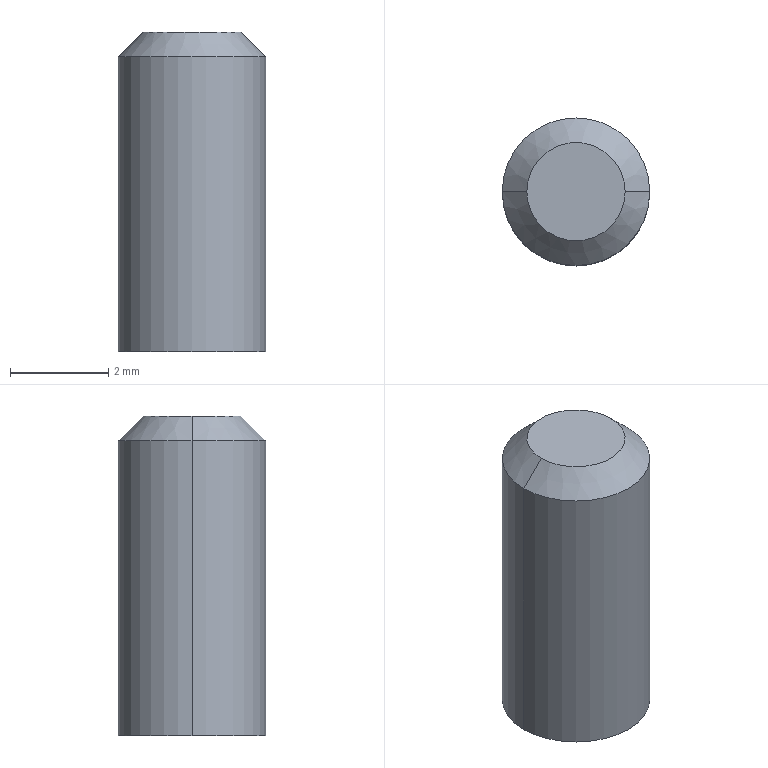Part | NX | 1 solid | 6 faces | box 3 x 3 x 6.5 mm | volume 44.899 mm3 | cylinder 2 | plane 2 | cone 2 | commonest cylinder face diameters 3 x2
STEP:
#1=CARTESIAN_POINT('',(-158.,178.7,-94.5));
#2=VERTEX_POINT('',#1);
#3=CARTESIAN_POINT('',(-161.,178.7,-94.5));
#4=VERTEX_POINT('',#3);
#5=CARTESIAN_POINT('',(-159.5,178.7,-94.5));
#6=DIRECTION('',(0.,0.,-1.));
#7=DIRECTION('',(-1.,0.,0.));
#8=AXIS2_PLACEMENT_3D('',#5,#6,#7);
#9=CIRCLE('',#8,1.5);
#10=EDGE_CURVE('',#2,#4,#9,.T.);
#11=ORIENTED_EDGE('',*,*,#10,.T.);
#12=CARTESIAN_POINT('',(-161.,178.7,-100.5));
#13=VERTEX_POINT('',#12);
#14=CARTESIAN_POINT('',(-161.,178.7,-100.5));
#15=DIRECTION('',(0.,0.,-1.));
#16=VECTOR('',#15,1000.);
#17=LINE('',#14,#16);
#18=EDGE_CURVE('',#13,#4,#17,.F.);
#19=ORIENTED_EDGE('',*,*,#18,.F.);
#20=CARTESIAN_POINT('',(-158.,178.7,-100.5));
#21=VERTEX_POINT('',#20);
#22=CARTESIAN_POINT('',(-159.5,178.7,-100.5));
#23=DIRECTION('',(0.,0.,-1.));
#24=DIRECTION('',(-1.,0.,0.));
#25=AXIS2_PLACEMENT_3D('',#22,#23,#24);
#26=CIRCLE('',#25,1.5);
#27=EDGE_CURVE('',#21,#13,#26,.T.);
#28=ORIENTED_EDGE('',*,*,#27,.F.);
#29=CARTESIAN_POINT('',(-158.,178.7,-100.5));
#30=DIRECTION('',(0.,0.,-1.));
#31=VECTOR('',#30,1000.);
#32=LINE('',#29,#31);
#33=EDGE_CURVE('',#21,#2,#32,.F.);
#34=ORIENTED_EDGE('',*,*,#33,.T.);
#35=EDGE_LOOP('',(#11,#19,#28,#34));
#36=FACE_BOUND('',#35,.T.);
#37=CARTESIAN_POINT('',(-159.5,178.7,-100.5));
#38=DIRECTION('',(0.,0.,-1.));
#39=DIRECTION('',(-1.,0.,0.));
#40=AXIS2_PLACEMENT_3D('',#37,#38,#39);
#41=CYLINDRICAL_SURFACE('',#40,1.5);
#42=ADVANCED_FACE('',(#36),#41,.T.);
#43=ORIENTED_EDGE('',*,*,#18,.T.);
#44=CARTESIAN_POINT('',(-159.5,178.7,-94.5));
#45=DIRECTION('',(0.,0.,-1.));
#46=DIRECTION('',(-1.,0.,0.));
#47=AXIS2_PLACEMENT_3D('',#44,#45,#46);
#48=CIRCLE('',#47,1.5);
#49=EDGE_CURVE('',#4,#2,#48,.T.);
#50=ORIENTED_EDGE('',*,*,#49,.T.);
#51=ORIENTED_EDGE('',*,*,#33,.F.);
#52=CARTESIAN_POINT('',(-159.5,178.7,-100.5));
#53=DIRECTION('',(0.,0.,-1.));
#54=DIRECTION('',(-1.,0.,0.));
#55=AXIS2_PLACEMENT_3D('',#52,#53,#54);
#56=CIRCLE('',#55,1.5);
#57=EDGE_CURVE('',#13,#21,#56,.T.);
#58=ORIENTED_EDGE('',*,*,#57,.F.);
#59=EDGE_LOOP('',(#43,#50,#51,#58));
#60=FACE_BOUND('',#59,.T.);
#61=CARTESIAN_POINT('',(-159.5,178.7,-100.5));
#62=DIRECTION('',(0.,0.,-1.));
#63=DIRECTION('',(-1.,0.,0.));
#64=AXIS2_PLACEMENT_3D('',#61,#62,#63);
#65=CYLINDRICAL_SURFACE('',#64,1.5);
#66=ADVANCED_FACE('',(#60),#65,.T.);
#67=CARTESIAN_POINT('',(-158.5,178.7,-94.));
#68=VERTEX_POINT('',#67);
#69=CARTESIAN_POINT('',(-160.5,178.7,-94.));
#70=VERTEX_POINT('',#69);
#71=CARTESIAN_POINT('',(-159.5,178.7,-94.));
#72=DIRECTION('',(0.,0.,-1.));
#73=DIRECTION('',(-1.,0.,0.));
#74=AXIS2_PLACEMENT_3D('',#71,#72,#73);
#75=CIRCLE('',#74,1.);
#76=EDGE_CURVE('',#68,#70,#75,.T.);
#77=ORIENTED_EDGE('',*,*,#76,.F.);
#78=CARTESIAN_POINT('',(-159.5,178.7,-94.));
#79=DIRECTION('',(0.,0.,-1.));
#80=DIRECTION('',(-1.,0.,0.));
#81=AXIS2_PLACEMENT_3D('',#78,#79,#80);
#82=CIRCLE('',#81,1.);
#83=EDGE_CURVE('',#70,#68,#82,.T.);
#84=ORIENTED_EDGE('',*,*,#83,.F.);
#85=EDGE_LOOP('',(#77,#84));
#86=FACE_BOUND('',#85,.T.);
#87=CARTESIAN_POINT('',(-154.068,179.819,-94.));
#88=DIRECTION('',(0.,0.,-1.));
#89=DIRECTION('',(-1.,0.,0.));
#90=AXIS2_PLACEMENT_3D('',#87,#88,#89);
#91=PLANE('',#90);
#92=ADVANCED_FACE('',(#86),#91,.F.);
#93=ORIENTED_EDGE('',*,*,#76,.T.);
#94=CARTESIAN_POINT('',(-160.5,178.7,-94.));
#95=DIRECTION('',(-0.7071,0.,-0.7071));
#96=VECTOR('',#95,1000.);
#97=LINE('',#94,#96);
#98=EDGE_CURVE('',#4,#70,#97,.F.);
#99=ORIENTED_EDGE('',*,*,#98,.F.);
#100=ORIENTED_EDGE('',*,*,#10,.F.);
#101=CARTESIAN_POINT('',(-158.5,178.7,-94.));
#102=DIRECTION('',(0.7071,0.,-0.7071));
#103=VECTOR('',#102,1000.);
#104=LINE('',#101,#103);
#105=EDGE_CURVE('',#2,#68,#104,.F.);
#106=ORIENTED_EDGE('',*,*,#105,.T.);
#107=EDGE_LOOP('',(#93,#99,#100,#106));
#108=FACE_BOUND('',#107,.T.);
#109=CARTESIAN_POINT('',(-159.5,178.7,-94.));
#110=DIRECTION('',(0.,0.,-1.));
#111=DIRECTION('',(-1.,0.,0.));
#112=AXIS2_PLACEMENT_3D('',#109,#110,#111);
#113=CONICAL_SURFACE('',#112,1.,0.7854);
#114=ADVANCED_FACE('',(#108),#113,.T.);
#115=ORIENTED_EDGE('',*,*,#98,.T.);
#116=ORIENTED_EDGE('',*,*,#83,.T.);
#117=ORIENTED_EDGE('',*,*,#105,.F.);
#118=ORIENTED_EDGE('',*,*,#49,.F.);
#119=EDGE_LOOP('',(#115,#116,#117,#118));
#120=FACE_BOUND('',#119,.T.);
#121=CARTESIAN_POINT('',(-159.5,178.7,-94.));
#122=DIRECTION('',(0.,0.,-1.));
#123=DIRECTION('',(-1.,0.,0.));
#124=AXIS2_PLACEMENT_3D('',#121,#122,#123);
#125=CONICAL_SURFACE('',#124,1.,0.7854);
#126=ADVANCED_FACE('',(#120),#125,.T.);
#127=ORIENTED_EDGE('',*,*,#27,.T.);
#128=ORIENTED_EDGE('',*,*,#57,.T.);
#129=EDGE_LOOP('',(#127,#128));
#130=FACE_BOUND('',#129,.T.);
#131=CARTESIAN_POINT('',(-154.068,179.819,-100.5));
#132=DIRECTION('',(0.,0.,-1.));
#133=DIRECTION('',(-1.,0.,0.));
#134=AXIS2_PLACEMENT_3D('',#131,#132,#133);
#135=PLANE('',#134);
#136=ADVANCED_FACE('',(#130),#135,.T.);
#137=CLOSED_SHELL('',(#42,#66,#92,#114,#126,#136));
#138=MANIFOLD_SOLID_BREP('',#137);
#139=(LENGTH_UNIT()NAMED_UNIT(*)SI_UNIT(.MILLI.,.METRE.));
#140=UNCERTAINTY_MEASURE_WITH_UNIT(LENGTH_MEASURE(0.00001),#139,'','');
#141=(NAMED_UNIT(*)PLANE_ANGLE_UNIT()SI_UNIT($,.RADIAN.));
#142=(NAMED_UNIT(*)SI_UNIT($,.STERADIAN.)SOLID_ANGLE_UNIT());
#143=(GEOMETRIC_REPRESENTATION_CONTEXT(3)GLOBAL_UNCERTAINTY_ASSIGNED_CONTEXT((#140))GLOBAL_UNIT_ASSIGNED_CONTEXT((#139,#141,#142))REPRESENTATION_CONTEXT('',''));
#144=ADVANCED_BREP_SHAPE_REPRESENTATION('',(#138),#143);